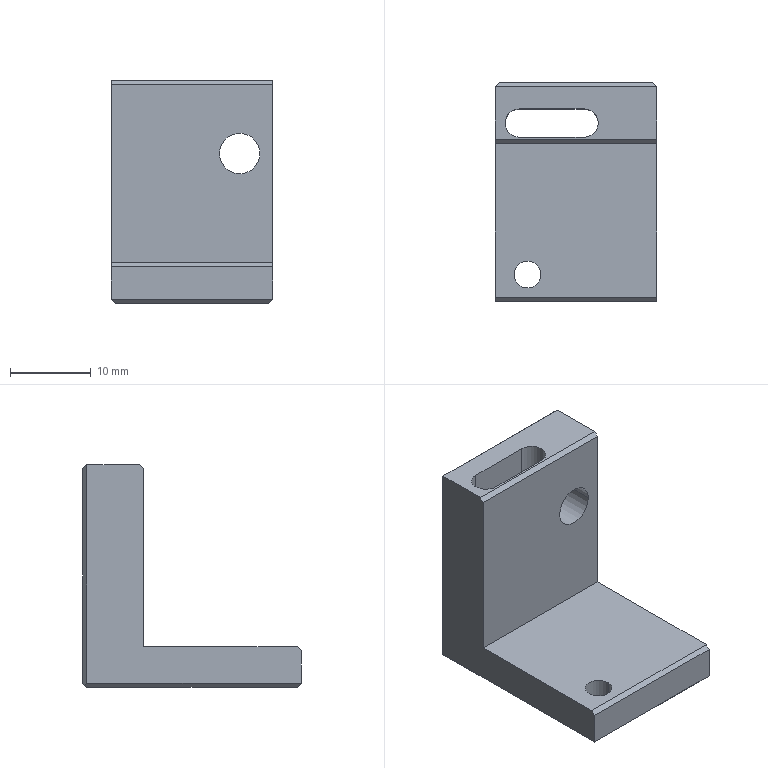Part | NX | 1 solid | 27 faces | box 20 x 27 x 27.5 mm | volume 4823 mm3 | plane 19 | cylinder 6 | cone 2 | commonest cylinder face diameters 3.3 x2 3.5 x2 5 x2
STEP:
#1=CARTESIAN_POINT('',(0.,9.5,-13.25));
#2=VERTEX_POINT('',#1);
#3=CARTESIAN_POINT('',(0.,9.5,13.75));
#4=VERTEX_POINT('',#3);
#5=CARTESIAN_POINT('',(0.,9.5,0.));
#6=DIRECTION('',(0.,0.,1.));
#7=VECTOR('',#6,1000.);
#8=LINE('',#5,#7);
#9=EDGE_CURVE('',#2,#4,#8,.T.);
#10=ORIENTED_EDGE('',*,*,#9,.F.);
#11=CARTESIAN_POINT('',(0.,-17.,-13.25));
#12=VERTEX_POINT('',#11);
#13=CARTESIAN_POINT('',(0.,0.,-13.25));
#14=DIRECTION('',(0.,1.,0.));
#15=VECTOR('',#14,1000.);
#16=LINE('',#13,#15);
#17=EDGE_CURVE('',#12,#2,#16,.T.);
#18=ORIENTED_EDGE('',*,*,#17,.F.);
#19=CARTESIAN_POINT('',(0.,-17.,-9.25));
#20=VERTEX_POINT('',#19);
#21=CARTESIAN_POINT('',(0.,-17.,0.));
#22=DIRECTION('',(0.,0.,1.));
#23=VECTOR('',#22,1000.);
#24=LINE('',#21,#23);
#25=EDGE_CURVE('',#12,#20,#24,.T.);
#26=ORIENTED_EDGE('',*,*,#25,.T.);
#27=CARTESIAN_POINT('',(0.,-16.5,-8.75));
#28=VERTEX_POINT('',#27);
#29=CARTESIAN_POINT('',(0.,-7.75,0.));
#30=DIRECTION('',(0.,-0.7071,-0.7071));
#31=VECTOR('',#30,1000.);
#32=LINE('',#29,#31);
#33=EDGE_CURVE('',#28,#20,#32,.T.);
#34=ORIENTED_EDGE('',*,*,#33,.F.);
#35=CARTESIAN_POINT('',(0.,2.5,-8.75));
#36=VERTEX_POINT('',#35);
#37=CARTESIAN_POINT('',(0.,0.,-8.75));
#38=DIRECTION('',(0.,1.,0.));
#39=VECTOR('',#38,1000.);
#40=LINE('',#37,#39);
#41=EDGE_CURVE('',#28,#36,#40,.T.);
#42=ORIENTED_EDGE('',*,*,#41,.T.);
#43=CARTESIAN_POINT('',(0.,2.5,13.25));
#44=VERTEX_POINT('',#43);
#45=CARTESIAN_POINT('',(0.,2.5,0.));
#46=DIRECTION('',(0.,0.,1.));
#47=VECTOR('',#46,1000.);
#48=LINE('',#45,#47);
#49=EDGE_CURVE('',#36,#44,#48,.T.);
#50=ORIENTED_EDGE('',*,*,#49,.T.);
#51=CARTESIAN_POINT('',(0.,3.,13.75));
#52=VERTEX_POINT('',#51);
#53=CARTESIAN_POINT('',(0.,-10.75,0.));
#54=DIRECTION('',(0.,0.7071,0.7071));
#55=VECTOR('',#54,1000.);
#56=LINE('',#53,#55);
#57=EDGE_CURVE('',#44,#52,#56,.T.);
#58=ORIENTED_EDGE('',*,*,#57,.T.);
#59=CARTESIAN_POINT('',(0.,0.,13.75));
#60=DIRECTION('',(0.,-1.,0.));
#61=VECTOR('',#60,1000.);
#62=LINE('',#59,#61);
#63=EDGE_CURVE('',#4,#52,#62,.T.);
#64=ORIENTED_EDGE('',*,*,#63,.F.);
#65=EDGE_LOOP('',(#10,#18,#26,#34,#42,#50,#58,#64));
#66=FACE_BOUND('',#65,.T.);
#67=CARTESIAN_POINT('',(0.,0.,0.));
#68=DIRECTION('',(-1.,0.,0.));
#69=DIRECTION('',(0.,0.,1.));
#70=AXIS2_PLACEMENT_3D('',#67,#68,#69);
#71=PLANE('',#70);
#72=ADVANCED_FACE('',(#66),#71,.T.);
#73=CARTESIAN_POINT('',(20.,3.,13.75));
#74=VERTEX_POINT('',#73);
#75=CARTESIAN_POINT('',(0.,3.,13.75));
#76=DIRECTION('',(-1.,0.,0.));
#77=VECTOR('',#76,1000.);
#78=LINE('',#75,#77);
#79=EDGE_CURVE('',#74,#52,#78,.T.);
#80=ORIENTED_EDGE('',*,*,#79,.F.);
#81=CARTESIAN_POINT('',(20.,9.5,13.75));
#82=VERTEX_POINT('',#81);
#83=CARTESIAN_POINT('',(20.,0.,13.75));
#84=DIRECTION('',(0.,-1.,0.));
#85=VECTOR('',#84,1000.);
#86=LINE('',#83,#85);
#87=EDGE_CURVE('',#82,#74,#86,.T.);
#88=ORIENTED_EDGE('',*,*,#87,.F.);
#89=CARTESIAN_POINT('',(0.,9.5,13.75));
#90=DIRECTION('',(-1.,0.,0.));
#91=VECTOR('',#90,1000.);
#92=LINE('',#89,#91);
#93=EDGE_CURVE('',#82,#4,#92,.T.);
#94=ORIENTED_EDGE('',*,*,#93,.T.);
#95=ORIENTED_EDGE('',*,*,#63,.T.);
#96=EDGE_LOOP('',(#80,#88,#94,#95));
#97=FACE_BOUND('',#96,.T.);
#98=CARTESIAN_POINT('',(11.,6.75,13.75));
#99=VERTEX_POINT('',#98);
#100=CARTESIAN_POINT('',(11.,3.25,13.75));
#101=VERTEX_POINT('',#100);
#102=CARTESIAN_POINT('',(11.,5.,13.75));
#103=DIRECTION('',(0.,0.,-1.));
#104=DIRECTION('',(1.,0.,0.));
#105=AXIS2_PLACEMENT_3D('',#102,#103,#104);
#106=CIRCLE('',#105,1.75);
#107=EDGE_CURVE('',#99,#101,#106,.T.);
#108=ORIENTED_EDGE('',*,*,#107,.T.);
#109=CARTESIAN_POINT('',(3.,3.25,13.75));
#110=VERTEX_POINT('',#109);
#111=CARTESIAN_POINT('',(0.,3.25,13.75));
#112=DIRECTION('',(-1.,0.,0.));
#113=VECTOR('',#112,1000.);
#114=LINE('',#111,#113);
#115=EDGE_CURVE('',#101,#110,#114,.T.);
#116=ORIENTED_EDGE('',*,*,#115,.T.);
#117=CARTESIAN_POINT('',(3.,6.75,13.75));
#118=VERTEX_POINT('',#117);
#119=CARTESIAN_POINT('',(3.,5.,13.75));
#120=DIRECTION('',(0.,0.,-1.));
#121=DIRECTION('',(1.,0.,0.));
#122=AXIS2_PLACEMENT_3D('',#119,#120,#121);
#123=CIRCLE('',#122,1.75);
#124=EDGE_CURVE('',#110,#118,#123,.T.);
#125=ORIENTED_EDGE('',*,*,#124,.T.);
#126=CARTESIAN_POINT('',(0.,6.75,13.75));
#127=DIRECTION('',(1.,0.,0.));
#128=VECTOR('',#127,1000.);
#129=LINE('',#126,#128);
#130=EDGE_CURVE('',#118,#99,#129,.T.);
#131=ORIENTED_EDGE('',*,*,#130,.T.);
#132=EDGE_LOOP('',(#108,#116,#125,#131));
#133=FACE_BOUND('',#132,.T.);
#134=CARTESIAN_POINT('',(0.,-17.,13.75));
#135=DIRECTION('',(0.,0.,-1.));
#136=DIRECTION('',(0.,-1.,0.));
#137=AXIS2_PLACEMENT_3D('',#134,#135,#136);
#138=PLANE('',#137);
#139=ADVANCED_FACE('',(#97,#133),#138,.F.);
#140=CARTESIAN_POINT('',(1.685,-13.7,-13.75));
#141=VERTEX_POINT('',#140);
#142=CARTESIAN_POINT('',(6.315,-13.7,-13.75));
#143=VERTEX_POINT('',#142);
#144=CARTESIAN_POINT('',(4.,-13.7,-13.75));
#145=DIRECTION('',(0.,0.,-1.));
#146=DIRECTION('',(-1.,0.,0.));
#147=AXIS2_PLACEMENT_3D('',#144,#145,#146);
#148=CIRCLE('',#147,2.315);
#149=EDGE_CURVE('',#141,#143,#148,.T.);
#150=ORIENTED_EDGE('',*,*,#149,.T.);
#151=CARTESIAN_POINT('',(5.65,-13.7,-13.366));
#152=VERTEX_POINT('',#151);
#153=CARTESIAN_POINT('',(5.65,-13.7,-13.366));
#154=DIRECTION('',(0.866,0.,-0.5));
#155=VECTOR('',#154,1000.);
#156=LINE('',#153,#155);
#157=EDGE_CURVE('',#143,#152,#156,.F.);
#158=ORIENTED_EDGE('',*,*,#157,.T.);
#159=CARTESIAN_POINT('',(2.35,-13.7,-13.366));
#160=VERTEX_POINT('',#159);
#161=CARTESIAN_POINT('',(4.,-13.7,-13.366));
#162=DIRECTION('',(0.,0.,-1.));
#163=DIRECTION('',(-1.,0.,0.));
#164=AXIS2_PLACEMENT_3D('',#161,#162,#163);
#165=CIRCLE('',#164,1.65);
#166=EDGE_CURVE('',#160,#152,#165,.T.);
#167=ORIENTED_EDGE('',*,*,#166,.F.);
#168=CARTESIAN_POINT('',(2.35,-13.7,-13.366));
#169=DIRECTION('',(-0.866,0.,-0.5));
#170=VECTOR('',#169,1000.);
#171=LINE('',#168,#170);
#172=EDGE_CURVE('',#141,#160,#171,.F.);
#173=ORIENTED_EDGE('',*,*,#172,.F.);
#174=EDGE_LOOP('',(#150,#158,#167,#173));
#175=FACE_BOUND('',#174,.T.);
#176=CARTESIAN_POINT('',(4.,-13.7,-13.366));
#177=DIRECTION('',(0.,0.,-1.));
#178=DIRECTION('',(-1.,0.,0.));
#179=AXIS2_PLACEMENT_3D('',#176,#177,#178);
#180=CONICAL_SURFACE('',#179,1.65,1.047);
#181=ADVANCED_FACE('',(#175),#180,.F.);
#182=CARTESIAN_POINT('',(20.,9.5,-13.25));
#183=VERTEX_POINT('',#182);
#184=CARTESIAN_POINT('',(20.,9.5,0.));
#185=DIRECTION('',(0.,0.,-1.));
#186=VECTOR('',#185,1000.);
#187=LINE('',#184,#186);
#188=EDGE_CURVE('',#82,#183,#187,.T.);
#189=ORIENTED_EDGE('',*,*,#188,.F.);
#190=ORIENTED_EDGE('',*,*,#87,.T.);
#191=CARTESIAN_POINT('',(20.,2.5,13.25));
#192=VERTEX_POINT('',#191);
#193=CARTESIAN_POINT('',(20.,-10.75,0.));
#194=DIRECTION('',(0.,0.7071,0.7071));
#195=VECTOR('',#194,1000.);
#196=LINE('',#193,#195);
#197=EDGE_CURVE('',#192,#74,#196,.T.);
#198=ORIENTED_EDGE('',*,*,#197,.F.);
#199=CARTESIAN_POINT('',(20.,2.5,-8.75));
#200=VERTEX_POINT('',#199);
#201=CARTESIAN_POINT('',(20.,2.5,0.));
#202=DIRECTION('',(0.,0.,1.));
#203=VECTOR('',#202,1000.);
#204=LINE('',#201,#203);
#205=EDGE_CURVE('',#200,#192,#204,.T.);
#206=ORIENTED_EDGE('',*,*,#205,.F.);
#207=CARTESIAN_POINT('',(20.,-16.5,-8.75));
#208=VERTEX_POINT('',#207);
#209=CARTESIAN_POINT('',(20.,0.,-8.75));
#210=DIRECTION('',(0.,1.,0.));
#211=VECTOR('',#210,1000.);
#212=LINE('',#209,#211);
#213=EDGE_CURVE('',#208,#200,#212,.T.);
#214=ORIENTED_EDGE('',*,*,#213,.F.);
#215=CARTESIAN_POINT('',(20.,-17.,-9.25));
#216=VERTEX_POINT('',#215);
#217=CARTESIAN_POINT('',(20.,-7.75,0.));
#218=DIRECTION('',(0.,-0.7071,-0.7071));
#219=VECTOR('',#218,1000.);
#220=LINE('',#217,#219);
#221=EDGE_CURVE('',#208,#216,#220,.T.);
#222=ORIENTED_EDGE('',*,*,#221,.T.);
#223=CARTESIAN_POINT('',(20.,-17.,-13.25));
#224=VERTEX_POINT('',#223);
#225=CARTESIAN_POINT('',(20.,-17.,0.));
#226=DIRECTION('',(0.,0.,1.));
#227=VECTOR('',#226,1000.);
#228=LINE('',#225,#227);
#229=EDGE_CURVE('',#224,#216,#228,.T.);
#230=ORIENTED_EDGE('',*,*,#229,.F.);
#231=CARTESIAN_POINT('',(20.,0.,-13.25));
#232=DIRECTION('',(0.,-1.,0.));
#233=VECTOR('',#232,1000.);
#234=LINE('',#231,#233);
#235=EDGE_CURVE('',#183,#224,#234,.T.);
#236=ORIENTED_EDGE('',*,*,#235,.F.);
#237=EDGE_LOOP('',(#189,#190,#198,#206,#214,#222,#230,#236));
#238=FACE_BOUND('',#237,.T.);
#239=CARTESIAN_POINT('',(20.,0.,0.));
#240=DIRECTION('',(-1.,0.,0.));
#241=DIRECTION('',(0.,0.,1.));
#242=AXIS2_PLACEMENT_3D('',#239,#240,#241);
#243=PLANE('',#242);
#244=ADVANCED_FACE('',(#238),#243,.F.);
#245=CARTESIAN_POINT('',(0.,-16.5,-8.75));
#246=DIRECTION('',(-1.,0.,0.));
#247=VECTOR('',#246,1000.);
#248=LINE('',#245,#247);
#249=EDGE_CURVE('',#208,#28,#248,.T.);
#250=ORIENTED_EDGE('',*,*,#249,.F.);
#251=ORIENTED_EDGE('',*,*,#213,.T.);
#252=CARTESIAN_POINT('',(0.,2.5,-8.75));
#253=DIRECTION('',(-1.,0.,0.));
#254=VECTOR('',#253,1000.);
#255=LINE('',#252,#254);
#256=EDGE_CURVE('',#200,#36,#255,.T.);
#257=ORIENTED_EDGE('',*,*,#256,.T.);
#258=ORIENTED_EDGE('',*,*,#41,.F.);
#259=EDGE_LOOP('',(#250,#251,#257,#258));
#260=FACE_BOUND('',#259,.T.);
#261=CARTESIAN_POINT('',(5.65,-13.7,-8.75));
#262=VERTEX_POINT('',#261);
#263=CARTESIAN_POINT('',(2.35,-13.7,-8.75));
#264=VERTEX_POINT('',#263);
#265=CARTESIAN_POINT('',(4.,-13.7,-8.75));
#266=DIRECTION('',(0.,0.,-1.));
#267=DIRECTION('',(-1.,0.,0.));
#268=AXIS2_PLACEMENT_3D('',#265,#266,#267);
#269=CIRCLE('',#268,1.65);
#270=EDGE_CURVE('',#262,#264,#269,.T.);
#271=ORIENTED_EDGE('',*,*,#270,.T.);
#272=CARTESIAN_POINT('',(4.,-13.7,-8.75));
#273=DIRECTION('',(0.,0.,-1.));
#274=DIRECTION('',(-1.,0.,0.));
#275=AXIS2_PLACEMENT_3D('',#272,#273,#274);
#276=CIRCLE('',#275,1.65);
#277=EDGE_CURVE('',#264,#262,#276,.T.);
#278=ORIENTED_EDGE('',*,*,#277,.T.);
#279=EDGE_LOOP('',(#271,#278));
#280=FACE_BOUND('',#279,.T.);
#281=CARTESIAN_POINT('',(0.,-17.,-8.75));
#282=DIRECTION('',(0.,0.,1.));
#283=DIRECTION('',(1.,0.,0.));
#284=AXIS2_PLACEMENT_3D('',#281,#282,#283);
#285=PLANE('',#284);
#286=ADVANCED_FACE('',(#260,#280),#285,.T.);
#287=CARTESIAN_POINT('',(0.,-17.,-9.25));
#288=DIRECTION('',(-1.,0.,0.));
#289=VECTOR('',#288,1000.);
#290=LINE('',#287,#289);
#291=EDGE_CURVE('',#216,#20,#290,.T.);
#292=ORIENTED_EDGE('',*,*,#291,.T.);
#293=ORIENTED_EDGE('',*,*,#25,.F.);
#294=CARTESIAN_POINT('',(0.,-17.,-13.25));
#295=DIRECTION('',(-1.,0.,0.));
#296=VECTOR('',#295,1000.);
#297=LINE('',#294,#296);
#298=EDGE_CURVE('',#224,#12,#297,.T.);
#299=ORIENTED_EDGE('',*,*,#298,.F.);
#300=ORIENTED_EDGE('',*,*,#229,.T.);
#301=EDGE_LOOP('',(#292,#293,#299,#300));
#302=FACE_BOUND('',#301,.T.);
#303=CARTESIAN_POINT('',(0.,-17.,-13.75));
#304=DIRECTION('',(0.,1.,0.));
#305=DIRECTION('',(1.,0.,0.));
#306=AXIS2_PLACEMENT_3D('',#303,#304,#305);
#307=PLANE('',#306);
#308=ADVANCED_FACE('',(#302),#307,.F.);
#309=CARTESIAN_POINT('',(0.5,10.,13.25));
#310=VERTEX_POINT('',#309);
#311=CARTESIAN_POINT('',(19.5,10.,13.25));
#312=VERTEX_POINT('',#311);
#313=CARTESIAN_POINT('',(0.,10.,13.25));
#314=DIRECTION('',(1.,0.,0.));
#315=VECTOR('',#314,1000.);
#316=LINE('',#313,#315);
#317=EDGE_CURVE('',#310,#312,#316,.T.);
#318=ORIENTED_EDGE('',*,*,#317,.T.);
#319=CARTESIAN_POINT('',(19.5,10.,-13.25));
#320=VERTEX_POINT('',#319);
#321=CARTESIAN_POINT('',(19.5,10.,0.));
#322=DIRECTION('',(0.,0.,1.));
#323=VECTOR('',#322,1000.);
#324=LINE('',#321,#323);
#325=EDGE_CURVE('',#320,#312,#324,.T.);
#326=ORIENTED_EDGE('',*,*,#325,.F.);
#327=CARTESIAN_POINT('',(0.5,10.,-13.25));
#328=VERTEX_POINT('',#327);
#329=CARTESIAN_POINT('',(0.,10.,-13.25));
#330=DIRECTION('',(1.,0.,0.));
#331=VECTOR('',#330,1000.);
#332=LINE('',#329,#331);
#333=EDGE_CURVE('',#328,#320,#332,.T.);
#334=ORIENTED_EDGE('',*,*,#333,.F.);
#335=CARTESIAN_POINT('',(0.5,10.,0.));
#336=DIRECTION('',(0.,0.,1.));
#337=VECTOR('',#336,1000.);
#338=LINE('',#335,#337);
#339=EDGE_CURVE('',#328,#310,#338,.T.);
#340=ORIENTED_EDGE('',*,*,#339,.T.);
#341=EDGE_LOOP('',(#318,#326,#334,#340));
#342=FACE_BOUND('',#341,.T.);
#343=CARTESIAN_POINT('',(18.4,10.,4.75));
#344=VERTEX_POINT('',#343);
#345=CARTESIAN_POINT('',(13.4,10.,4.75));
#346=VERTEX_POINT('',#345);
#347=CARTESIAN_POINT('',(15.9,10.,4.75));
#348=DIRECTION('',(0.,1.,0.));
#349=DIRECTION('',(-1.,0.,0.));
#350=AXIS2_PLACEMENT_3D('',#347,#348,#349);
#351=CIRCLE('',#350,2.5);
#352=EDGE_CURVE('',#344,#346,#351,.T.);
#353=ORIENTED_EDGE('',*,*,#352,.F.);
#354=CARTESIAN_POINT('',(15.9,10.,4.75));
#355=DIRECTION('',(0.,1.,0.));
#356=DIRECTION('',(-1.,0.,0.));
#357=AXIS2_PLACEMENT_3D('',#354,#355,#356);
#358=CIRCLE('',#357,2.5);
#359=EDGE_CURVE('',#346,#344,#358,.T.);
#360=ORIENTED_EDGE('',*,*,#359,.F.);
#361=EDGE_LOOP('',(#353,#360));
#362=FACE_BOUND('',#361,.T.);
#363=CARTESIAN_POINT('',(0.,10.,13.75));
#364=DIRECTION('',(0.,-1.,0.));
#365=DIRECTION('',(0.,0.,-1.));
#366=AXIS2_PLACEMENT_3D('',#363,#364,#365);
#367=PLANE('',#366);
#368=ADVANCED_FACE('',(#342,#362),#367,.F.);
#369=CARTESIAN_POINT('',(0.,2.5,13.25));
#370=DIRECTION('',(-1.,0.,0.));
#371=VECTOR('',#370,1000.);
#372=LINE('',#369,#371);
#373=EDGE_CURVE('',#192,#44,#372,.T.);
#374=ORIENTED_EDGE('',*,*,#373,.T.);
#375=ORIENTED_EDGE('',*,*,#49,.F.);
#376=ORIENTED_EDGE('',*,*,#256,.F.);
#377=ORIENTED_EDGE('',*,*,#205,.T.);
#378=EDGE_LOOP('',(#374,#375,#376,#377));
#379=FACE_BOUND('',#378,.T.);
#380=CARTESIAN_POINT('',(18.4,2.5,4.75));
#381=VERTEX_POINT('',#380);
#382=CARTESIAN_POINT('',(13.4,2.5,4.75));
#383=VERTEX_POINT('',#382);
#384=CARTESIAN_POINT('',(15.9,2.5,4.75));
#385=DIRECTION('',(0.,1.,0.));
#386=DIRECTION('',(1.,0.,0.));
#387=AXIS2_PLACEMENT_3D('',#384,#385,#386);
#388=CIRCLE('',#387,2.5);
#389=EDGE_CURVE('',#381,#383,#388,.T.);
#390=ORIENTED_EDGE('',*,*,#389,.T.);
#391=CARTESIAN_POINT('',(15.9,2.5,4.75));
#392=DIRECTION('',(0.,1.,0.));
#393=DIRECTION('',(1.,0.,0.));
#394=AXIS2_PLACEMENT_3D('',#391,#392,#393);
#395=CIRCLE('',#394,2.5);
#396=EDGE_CURVE('',#383,#381,#395,.T.);
#397=ORIENTED_EDGE('',*,*,#396,.T.);
#398=EDGE_LOOP('',(#390,#397));
#399=FACE_BOUND('',#398,.T.);
#400=CARTESIAN_POINT('',(0.,2.5,-8.75));
#401=DIRECTION('',(0.,-1.,0.));
#402=DIRECTION('',(0.,0.,-1.));
#403=AXIS2_PLACEMENT_3D('',#400,#401,#402);
#404=PLANE('',#403);
#405=ADVANCED_FACE('',(#379,#399),#404,.T.);
#406=CARTESIAN_POINT('',(19.5,9.5,-13.75));
#407=VERTEX_POINT('',#406);
#408=CARTESIAN_POINT('',(0.5,9.5,-13.75));
#409=VERTEX_POINT('',#408);
#410=CARTESIAN_POINT('',(0.,9.5,-13.75));
#411=DIRECTION('',(-1.,0.,0.));
#412=VECTOR('',#411,1000.);
#413=LINE('',#410,#412);
#414=EDGE_CURVE('',#407,#409,#413,.T.);
#415=ORIENTED_EDGE('',*,*,#414,.F.);
#416=CARTESIAN_POINT('',(19.5,-16.5,-13.75));
#417=VERTEX_POINT('',#416);
#418=CARTESIAN_POINT('',(19.5,0.,-13.75));
#419=DIRECTION('',(0.,1.,0.));
#420=VECTOR('',#419,1000.);
#421=LINE('',#418,#420);
#422=EDGE_CURVE('',#417,#407,#421,.T.);
#423=ORIENTED_EDGE('',*,*,#422,.F.);
#424=CARTESIAN_POINT('',(0.5,-16.5,-13.75));
#425=VERTEX_POINT('',#424);
#426=CARTESIAN_POINT('',(0.,-16.5,-13.75));
#427=DIRECTION('',(1.,0.,0.));
#428=VECTOR('',#427,1000.);
#429=LINE('',#426,#428);
#430=EDGE_CURVE('',#425,#417,#429,.T.);
#431=ORIENTED_EDGE('',*,*,#430,.F.);
#432=CARTESIAN_POINT('',(0.5,0.,-13.75));
#433=DIRECTION('',(0.,1.,0.));
#434=VECTOR('',#433,1000.);
#435=LINE('',#432,#434);
#436=EDGE_CURVE('',#425,#409,#435,.T.);
#437=ORIENTED_EDGE('',*,*,#436,.T.);
#438=EDGE_LOOP('',(#415,#423,#431,#437));
#439=FACE_BOUND('',#438,.T.);
#440=CARTESIAN_POINT('',(3.,6.75,-13.75));
#441=VERTEX_POINT('',#440);
#442=CARTESIAN_POINT('',(11.,6.75,-13.75));
#443=VERTEX_POINT('',#442);
#444=CARTESIAN_POINT('',(0.,6.75,-13.75));
#445=DIRECTION('',(1.,0.,0.));
#446=VECTOR('',#445,1000.);
#447=LINE('',#444,#446);
#448=EDGE_CURVE('',#441,#443,#447,.T.);
#449=ORIENTED_EDGE('',*,*,#448,.F.);
#450=CARTESIAN_POINT('',(3.,3.25,-13.75));
#451=VERTEX_POINT('',#450);
#452=CARTESIAN_POINT('',(3.,5.,-13.75));
#453=DIRECTION('',(0.,0.,-1.));
#454=DIRECTION('',(1.,0.,0.));
#455=AXIS2_PLACEMENT_3D('',#452,#453,#454);
#456=CIRCLE('',#455,1.75);
#457=EDGE_CURVE('',#451,#441,#456,.T.);
#458=ORIENTED_EDGE('',*,*,#457,.F.);
#459=CARTESIAN_POINT('',(11.,3.25,-13.75));
#460=VERTEX_POINT('',#459);
#461=CARTESIAN_POINT('',(0.,3.25,-13.75));
#462=DIRECTION('',(-1.,0.,0.));
#463=VECTOR('',#462,1000.);
#464=LINE('',#461,#463);
#465=EDGE_CURVE('',#460,#451,#464,.T.);
#466=ORIENTED_EDGE('',*,*,#465,.F.);
#467=CARTESIAN_POINT('',(11.,5.,-13.75));
#468=DIRECTION('',(0.,0.,-1.));
#469=DIRECTION('',(-1.,0.,0.));
#470=AXIS2_PLACEMENT_3D('',#467,#468,#469);
#471=CIRCLE('',#470,1.75);
#472=EDGE_CURVE('',#443,#460,#471,.T.);
#473=ORIENTED_EDGE('',*,*,#472,.F.);
#474=EDGE_LOOP('',(#449,#458,#466,#473));
#475=FACE_BOUND('',#474,.T.);
#476=ORIENTED_EDGE('',*,*,#149,.F.);
#477=CARTESIAN_POINT('',(4.,-13.7,-13.75));
#478=DIRECTION('',(0.,0.,-1.));
#479=DIRECTION('',(-1.,0.,0.));
#480=AXIS2_PLACEMENT_3D('',#477,#478,#479);
#481=CIRCLE('',#480,2.315);
#482=EDGE_CURVE('',#143,#141,#481,.T.);
#483=ORIENTED_EDGE('',*,*,#482,.F.);
#484=EDGE_LOOP('',(#476,#483));
#485=FACE_BOUND('',#484,.T.);
#486=CARTESIAN_POINT('',(0.,10.,-13.75));
#487=DIRECTION('',(0.,0.,1.));
#488=DIRECTION('',(1.,0.,0.));
#489=AXIS2_PLACEMENT_3D('',#486,#487,#488);
#490=PLANE('',#489);
#491=ADVANCED_FACE('',(#439,#475,#485),#490,.F.);
#492=ORIENTED_EDGE('',*,*,#107,.F.);
#493=CARTESIAN_POINT('',(11.,6.75,-13.75));
#494=DIRECTION('',(0.,0.,-1.));
#495=VECTOR('',#494,1000.);
#496=LINE('',#493,#495);
#497=EDGE_CURVE('',#99,#443,#496,.T.);
#498=ORIENTED_EDGE('',*,*,#497,.T.);
#499=ORIENTED_EDGE('',*,*,#472,.T.);
#500=CARTESIAN_POINT('',(11.,3.25,-13.75));
#501=DIRECTION('',(0.,0.,-1.));
#502=VECTOR('',#501,1000.);
#503=LINE('',#500,#502);
#504=EDGE_CURVE('',#101,#460,#503,.T.);
#505=ORIENTED_EDGE('',*,*,#504,.F.);
#506=EDGE_LOOP('',(#492,#498,#499,#505));
#507=FACE_BOUND('',#506,.T.);
#508=CARTESIAN_POINT('',(11.,5.,-13.75));
#509=DIRECTION('',(0.,0.,-1.));
#510=DIRECTION('',(-1.,0.,0.));
#511=AXIS2_PLACEMENT_3D('',#508,#509,#510);
#512=CYLINDRICAL_SURFACE('',#511,1.75);
#513=ADVANCED_FACE('',(#507),#512,.F.);
#514=ORIENTED_EDGE('',*,*,#352,.T.);
#515=CARTESIAN_POINT('',(13.4,10.,4.75));
#516=DIRECTION('',(0.,1.,0.));
#517=VECTOR('',#516,1000.);
#518=LINE('',#515,#517);
#519=EDGE_CURVE('',#383,#346,#518,.T.);
#520=ORIENTED_EDGE('',*,*,#519,.F.);
#521=ORIENTED_EDGE('',*,*,#389,.F.);
#522=CARTESIAN_POINT('',(18.4,10.,4.75));
#523=DIRECTION('',(0.,1.,0.));
#524=VECTOR('',#523,1000.);
#525=LINE('',#522,#524);
#526=EDGE_CURVE('',#381,#344,#525,.T.);
#527=ORIENTED_EDGE('',*,*,#526,.T.);
#528=EDGE_LOOP('',(#514,#520,#521,#527));
#529=FACE_BOUND('',#528,.T.);
#530=CARTESIAN_POINT('',(15.9,10.,4.75));
#531=DIRECTION('',(0.,1.,0.));
#532=DIRECTION('',(1.,0.,0.));
#533=AXIS2_PLACEMENT_3D('',#530,#531,#532);
#534=CYLINDRICAL_SURFACE('',#533,2.5);
#535=ADVANCED_FACE('',(#529),#534,.F.);
#536=ORIENTED_EDGE('',*,*,#414,.T.);
#537=CARTESIAN_POINT('',(0.25,9.75,-13.5));
#538=VERTEX_POINT('',#537);
#539=CARTESIAN_POINT('',(-13.25,23.25,0.));
#540=DIRECTION('',(0.5774,-0.5774,-0.5774));
#541=VECTOR('',#540,1000.);
#542=LINE('',#539,#541);
#543=EDGE_CURVE('',#538,#409,#542,.T.);
#544=ORIENTED_EDGE('',*,*,#543,.F.);
#545=CARTESIAN_POINT('',(13.75,23.25,0.));
#546=DIRECTION('',(-0.5774,-0.5774,-0.5774));
#547=VECTOR('',#546,1000.);
#548=LINE('',#545,#547);
#549=EDGE_CURVE('',#328,#538,#548,.T.);
#550=ORIENTED_EDGE('',*,*,#549,.F.);
#551=ORIENTED_EDGE('',*,*,#333,.T.);
#552=CARTESIAN_POINT('',(19.75,9.75,-13.5));
#553=VERTEX_POINT('',#552);
#554=CARTESIAN_POINT('',(6.25,23.25,0.));
#555=DIRECTION('',(0.5774,-0.5774,-0.5774));
#556=VECTOR('',#555,1000.);
#557=LINE('',#554,#556);
#558=EDGE_CURVE('',#320,#553,#557,.T.);
#559=ORIENTED_EDGE('',*,*,#558,.T.);
#560=CARTESIAN_POINT('',(33.25,23.25,0.));
#561=DIRECTION('',(-0.5774,-0.5774,-0.5774));
#562=VECTOR('',#561,1000.);
#563=LINE('',#560,#562);
#564=EDGE_CURVE('',#553,#407,#563,.T.);
#565=ORIENTED_EDGE('',*,*,#564,.T.);
#566=EDGE_LOOP('',(#536,#544,#550,#551,#559,#565));
#567=FACE_BOUND('',#566,.T.);
#568=CARTESIAN_POINT('',(10.,9.75,-13.5));
#569=DIRECTION('',(0.,-0.7071,0.7071));
#570=DIRECTION('',(-1.,0.,0.));
#571=AXIS2_PLACEMENT_3D('',#568,#569,#570);
#572=PLANE('',#571);
#573=ADVANCED_FACE('',(#567),#572,.F.);
#574=ORIENTED_EDGE('',*,*,#166,.T.);
#575=CARTESIAN_POINT('',(5.65,-13.7,-13.75));
#576=DIRECTION('',(0.,0.,-1.));
#577=VECTOR('',#576,1000.);
#578=LINE('',#575,#577);
#579=EDGE_CURVE('',#262,#152,#578,.T.);
#580=ORIENTED_EDGE('',*,*,#579,.F.);
#581=ORIENTED_EDGE('',*,*,#277,.F.);
#582=CARTESIAN_POINT('',(2.35,-13.7,-13.75));
#583=DIRECTION('',(0.,0.,-1.));
#584=VECTOR('',#583,1000.);
#585=LINE('',#582,#584);
#586=EDGE_CURVE('',#264,#160,#585,.T.);
#587=ORIENTED_EDGE('',*,*,#586,.T.);
#588=EDGE_LOOP('',(#574,#580,#581,#587));
#589=FACE_BOUND('',#588,.T.);
#590=CARTESIAN_POINT('',(4.,-13.7,-13.75));
#591=DIRECTION('',(0.,0.,-1.));
#592=DIRECTION('',(-1.,0.,0.));
#593=AXIS2_PLACEMENT_3D('',#590,#591,#592);
#594=CYLINDRICAL_SURFACE('',#593,1.65);
#595=ADVANCED_FACE('',(#589),#594,.F.);
#596=ORIENTED_EDGE('',*,*,#188,.T.);
#597=CARTESIAN_POINT('',(33.25,-3.75,0.));
#598=DIRECTION('',(-0.5774,0.5774,-0.5774));
#599=VECTOR('',#598,1000.);
#600=LINE('',#597,#599);
#601=EDGE_CURVE('',#183,#553,#600,.T.);
#602=ORIENTED_EDGE('',*,*,#601,.T.);
#603=ORIENTED_EDGE('',*,*,#558,.F.);
#604=ORIENTED_EDGE('',*,*,#325,.T.);
#605=CARTESIAN_POINT('',(6.25,23.25,0.));
#606=DIRECTION('',(-0.5774,0.5774,-0.5774));
#607=VECTOR('',#606,1000.);
#608=LINE('',#605,#607);
#609=EDGE_CURVE('',#82,#312,#608,.T.);
#610=ORIENTED_EDGE('',*,*,#609,.F.);
#611=EDGE_LOOP('',(#596,#602,#603,#604,#610));
#612=FACE_BOUND('',#611,.T.);
#613=CARTESIAN_POINT('',(19.75,9.75,0.));
#614=DIRECTION('',(-0.7071,-0.7071,0.));
#615=DIRECTION('',(-0.7071,0.7071,0.));
#616=AXIS2_PLACEMENT_3D('',#613,#614,#615);
#617=PLANE('',#616);
#618=ADVANCED_FACE('',(#612),#617,.F.);
#619=ORIENTED_EDGE('',*,*,#9,.T.);
#620=CARTESIAN_POINT('',(13.75,23.25,0.));
#621=DIRECTION('',(0.5774,0.5774,-0.5774));
#622=VECTOR('',#621,1000.);
#623=LINE('',#620,#622);
#624=EDGE_CURVE('',#4,#310,#623,.T.);
#625=ORIENTED_EDGE('',*,*,#624,.T.);
#626=ORIENTED_EDGE('',*,*,#339,.F.);
#627=ORIENTED_EDGE('',*,*,#549,.T.);
#628=CARTESIAN_POINT('',(-13.25,-3.75,0.));
#629=DIRECTION('',(-0.5774,-0.5774,0.5774));
#630=VECTOR('',#629,1000.);
#631=LINE('',#628,#630);
#632=EDGE_CURVE('',#538,#2,#631,.T.);
#633=ORIENTED_EDGE('',*,*,#632,.T.);
#634=EDGE_LOOP('',(#619,#625,#626,#627,#633));
#635=FACE_BOUND('',#634,.T.);
#636=CARTESIAN_POINT('',(0.25,9.75,0.));
#637=DIRECTION('',(-0.7071,0.7071,0.));
#638=DIRECTION('',(0.,0.,1.));
#639=AXIS2_PLACEMENT_3D('',#636,#637,#638);
#640=PLANE('',#639);
#641=ADVANCED_FACE('',(#635),#640,.T.);
#642=ORIENTED_EDGE('',*,*,#422,.T.);
#643=ORIENTED_EDGE('',*,*,#564,.F.);
#644=ORIENTED_EDGE('',*,*,#601,.F.);
#645=ORIENTED_EDGE('',*,*,#235,.T.);
#646=CARTESIAN_POINT('',(33.25,-30.25,0.));
#647=DIRECTION('',(-0.5774,0.5774,-0.5774));
#648=VECTOR('',#647,1000.);
#649=LINE('',#646,#648);
#650=EDGE_CURVE('',#224,#417,#649,.T.);
#651=ORIENTED_EDGE('',*,*,#650,.T.);
#652=EDGE_LOOP('',(#642,#643,#644,#645,#651));
#653=FACE_BOUND('',#652,.T.);
#654=CARTESIAN_POINT('',(19.75,-3.5,-13.5));
#655=DIRECTION('',(-0.7071,0.,0.7071));
#656=DIRECTION('',(0.,1.,0.));
#657=AXIS2_PLACEMENT_3D('',#654,#655,#656);
#658=PLANE('',#657);
#659=ADVANCED_FACE('',(#653),#658,.F.);
#660=ORIENTED_EDGE('',*,*,#436,.F.);
#661=CARTESIAN_POINT('',(-13.25,-30.25,0.));
#662=DIRECTION('',(0.5774,0.5774,-0.5774));
#663=VECTOR('',#662,1000.);
#664=LINE('',#661,#663);
#665=EDGE_CURVE('',#12,#425,#664,.T.);
#666=ORIENTED_EDGE('',*,*,#665,.F.);
#667=ORIENTED_EDGE('',*,*,#17,.T.);
#668=ORIENTED_EDGE('',*,*,#632,.F.);
#669=ORIENTED_EDGE('',*,*,#543,.T.);
#670=EDGE_LOOP('',(#660,#666,#667,#668,#669));
#671=FACE_BOUND('',#670,.T.);
#672=CARTESIAN_POINT('',(0.25,-3.5,-13.5));
#673=DIRECTION('',(-0.7071,0.,-0.7071));
#674=DIRECTION('',(-0.7071,0.,0.7071));
#675=AXIS2_PLACEMENT_3D('',#672,#673,#674);
#676=PLANE('',#675);
#677=ADVANCED_FACE('',(#671),#676,.T.);
#678=ORIENTED_EDGE('',*,*,#430,.T.);
#679=ORIENTED_EDGE('',*,*,#650,.F.);
#680=ORIENTED_EDGE('',*,*,#298,.T.);
#681=ORIENTED_EDGE('',*,*,#665,.T.);
#682=EDGE_LOOP('',(#678,#679,#680,#681));
#683=FACE_BOUND('',#682,.T.);
#684=CARTESIAN_POINT('',(10.,-16.75,-13.5));
#685=DIRECTION('',(0.,0.7071,0.7071));
#686=DIRECTION('',(1.,0.,0.));
#687=AXIS2_PLACEMENT_3D('',#684,#685,#686);
#688=PLANE('',#687);
#689=ADVANCED_FACE('',(#683),#688,.F.);
#690=ORIENTED_EDGE('',*,*,#249,.T.);
#691=ORIENTED_EDGE('',*,*,#33,.T.);
#692=ORIENTED_EDGE('',*,*,#291,.F.);
#693=ORIENTED_EDGE('',*,*,#221,.F.);
#694=EDGE_LOOP('',(#690,#691,#692,#693));
#695=FACE_BOUND('',#694,.T.);
#696=CARTESIAN_POINT('',(10.,-16.75,-9.));
#697=DIRECTION('',(0.,-0.7071,0.7071));
#698=DIRECTION('',(-1.,0.,0.));
#699=AXIS2_PLACEMENT_3D('',#696,#697,#698);
#700=PLANE('',#699);
#701=ADVANCED_FACE('',(#695),#700,.T.);
#702=ORIENTED_EDGE('',*,*,#373,.F.);
#703=ORIENTED_EDGE('',*,*,#197,.T.);
#704=ORIENTED_EDGE('',*,*,#79,.T.);
#705=ORIENTED_EDGE('',*,*,#57,.F.);
#706=EDGE_LOOP('',(#702,#703,#704,#705));
#707=FACE_BOUND('',#706,.T.);
#708=CARTESIAN_POINT('',(10.,2.75,13.5));
#709=DIRECTION('',(0.,0.7071,-0.7071));
#710=DIRECTION('',(-1.,0.,0.));
#711=AXIS2_PLACEMENT_3D('',#708,#709,#710);
#712=PLANE('',#711);
#713=ADVANCED_FACE('',(#707),#712,.F.);
#714=ORIENTED_EDGE('',*,*,#317,.F.);
#715=ORIENTED_EDGE('',*,*,#624,.F.);
#716=ORIENTED_EDGE('',*,*,#93,.F.);
#717=ORIENTED_EDGE('',*,*,#609,.T.);
#718=EDGE_LOOP('',(#714,#715,#716,#717));
#719=FACE_BOUND('',#718,.T.);
#720=CARTESIAN_POINT('',(10.,9.75,13.5));
#721=DIRECTION('',(0.,0.7071,0.7071));
#722=DIRECTION('',(1.,0.,0.));
#723=AXIS2_PLACEMENT_3D('',#720,#721,#722);
#724=PLANE('',#723);
#725=ADVANCED_FACE('',(#719),#724,.T.);
#726=ORIENTED_EDGE('',*,*,#115,.F.);
#727=ORIENTED_EDGE('',*,*,#504,.T.);
#728=ORIENTED_EDGE('',*,*,#465,.T.);
#729=CARTESIAN_POINT('',(3.,3.25,16.5));
#730=DIRECTION('',(0.,0.,-1.));
#731=VECTOR('',#730,1000.);
#732=LINE('',#729,#731);
#733=EDGE_CURVE('',#110,#451,#732,.T.);
#734=ORIENTED_EDGE('',*,*,#733,.F.);
#735=EDGE_LOOP('',(#726,#727,#728,#734));
#736=FACE_BOUND('',#735,.T.);
#737=CARTESIAN_POINT('',(3.,3.25,16.5));
#738=DIRECTION('',(0.,-1.,0.));
#739=DIRECTION('',(0.,0.,-1.));
#740=AXIS2_PLACEMENT_3D('',#737,#738,#739);
#741=PLANE('',#740);
#742=ADVANCED_FACE('',(#736),#741,.F.);
#743=ORIENTED_EDGE('',*,*,#457,.T.);
#744=CARTESIAN_POINT('',(3.,6.75,16.5));
#745=DIRECTION('',(0.,0.,-1.));
#746=VECTOR('',#745,1000.);
#747=LINE('',#744,#746);
#748=EDGE_CURVE('',#118,#441,#747,.T.);
#749=ORIENTED_EDGE('',*,*,#748,.F.);
#750=ORIENTED_EDGE('',*,*,#124,.F.);
#751=ORIENTED_EDGE('',*,*,#733,.T.);
#752=EDGE_LOOP('',(#743,#749,#750,#751));
#753=FACE_BOUND('',#752,.T.);
#754=CARTESIAN_POINT('',(3.,5.,16.5));
#755=DIRECTION('',(0.,0.,-1.));
#756=DIRECTION('',(1.,0.,0.));
#757=AXIS2_PLACEMENT_3D('',#754,#755,#756);
#758=CYLINDRICAL_SURFACE('',#757,1.75);
#759=ADVANCED_FACE('',(#753),#758,.F.);
#760=ORIENTED_EDGE('',*,*,#130,.F.);
#761=ORIENTED_EDGE('',*,*,#748,.T.);
#762=ORIENTED_EDGE('',*,*,#448,.T.);
#763=ORIENTED_EDGE('',*,*,#497,.F.);
#764=EDGE_LOOP('',(#760,#761,#762,#763));
#765=FACE_BOUND('',#764,.T.);
#766=CARTESIAN_POINT('',(11.,6.75,16.5));
#767=DIRECTION('',(0.,1.,0.));
#768=DIRECTION('',(1.,0.,0.));
#769=AXIS2_PLACEMENT_3D('',#766,#767,#768);
#770=PLANE('',#769);
#771=ADVANCED_FACE('',(#765),#770,.F.);
#772=ORIENTED_EDGE('',*,*,#270,.F.);
#773=ORIENTED_EDGE('',*,*,#579,.T.);
#774=CARTESIAN_POINT('',(4.,-13.7,-13.366));
#775=DIRECTION('',(0.,0.,-1.));
#776=DIRECTION('',(-1.,0.,0.));
#777=AXIS2_PLACEMENT_3D('',#774,#775,#776);
#778=CIRCLE('',#777,1.65);
#779=EDGE_CURVE('',#152,#160,#778,.T.);
#780=ORIENTED_EDGE('',*,*,#779,.T.);
#781=ORIENTED_EDGE('',*,*,#586,.F.);
#782=EDGE_LOOP('',(#772,#773,#780,#781));
#783=FACE_BOUND('',#782,.T.);
#784=CARTESIAN_POINT('',(4.,-13.7,-13.75));
#785=DIRECTION('',(0.,0.,-1.));
#786=DIRECTION('',(-1.,0.,0.));
#787=AXIS2_PLACEMENT_3D('',#784,#785,#786);
#788=CYLINDRICAL_SURFACE('',#787,1.65);
#789=ADVANCED_FACE('',(#783),#788,.F.);
#790=ORIENTED_EDGE('',*,*,#526,.F.);
#791=ORIENTED_EDGE('',*,*,#396,.F.);
#792=ORIENTED_EDGE('',*,*,#519,.T.);
#793=ORIENTED_EDGE('',*,*,#359,.T.);
#794=EDGE_LOOP('',(#790,#791,#792,#793));
#795=FACE_BOUND('',#794,.T.);
#796=CARTESIAN_POINT('',(15.9,10.,4.75));
#797=DIRECTION('',(0.,1.,0.));
#798=DIRECTION('',(1.,0.,0.));
#799=AXIS2_PLACEMENT_3D('',#796,#797,#798);
#800=CYLINDRICAL_SURFACE('',#799,2.5);
#801=ADVANCED_FACE('',(#795),#800,.F.);
#802=ORIENTED_EDGE('',*,*,#172,.T.);
#803=ORIENTED_EDGE('',*,*,#779,.F.);
#804=ORIENTED_EDGE('',*,*,#157,.F.);
#805=ORIENTED_EDGE('',*,*,#482,.T.);
#806=EDGE_LOOP('',(#802,#803,#804,#805));
#807=FACE_BOUND('',#806,.T.);
#808=CARTESIAN_POINT('',(4.,-13.7,-13.366));
#809=DIRECTION('',(0.,0.,-1.));
#810=DIRECTION('',(-1.,0.,0.));
#811=AXIS2_PLACEMENT_3D('',#808,#809,#810);
#812=CONICAL_SURFACE('',#811,1.65,1.047);
#813=ADVANCED_FACE('',(#807),#812,.F.);
#814=CLOSED_SHELL('',(#72,#139,#181,#244,#286,#308,#368,#405,#491,#513,#535,#573,#595,#618,#641,#659,#677,#689,#701,#713,#725,#742,#759,#771,#789,#801,#813));
#815=MANIFOLD_SOLID_BREP('',#814);
#816=(LENGTH_UNIT()NAMED_UNIT(*)SI_UNIT(.MILLI.,.METRE.));
#817=UNCERTAINTY_MEASURE_WITH_UNIT(LENGTH_MEASURE(0.00001),#816,'','');
#818=(NAMED_UNIT(*)PLANE_ANGLE_UNIT()SI_UNIT($,.RADIAN.));
#819=(NAMED_UNIT(*)SI_UNIT($,.STERADIAN.)SOLID_ANGLE_UNIT());
#820=(GEOMETRIC_REPRESENTATION_CONTEXT(3)GLOBAL_UNCERTAINTY_ASSIGNED_CONTEXT((#817))GLOBAL_UNIT_ASSIGNED_CONTEXT((#816,#818,#819))REPRESENTATION_CONTEXT('',''));
#821=ADVANCED_BREP_SHAPE_REPRESENTATION('',(#815),#820);